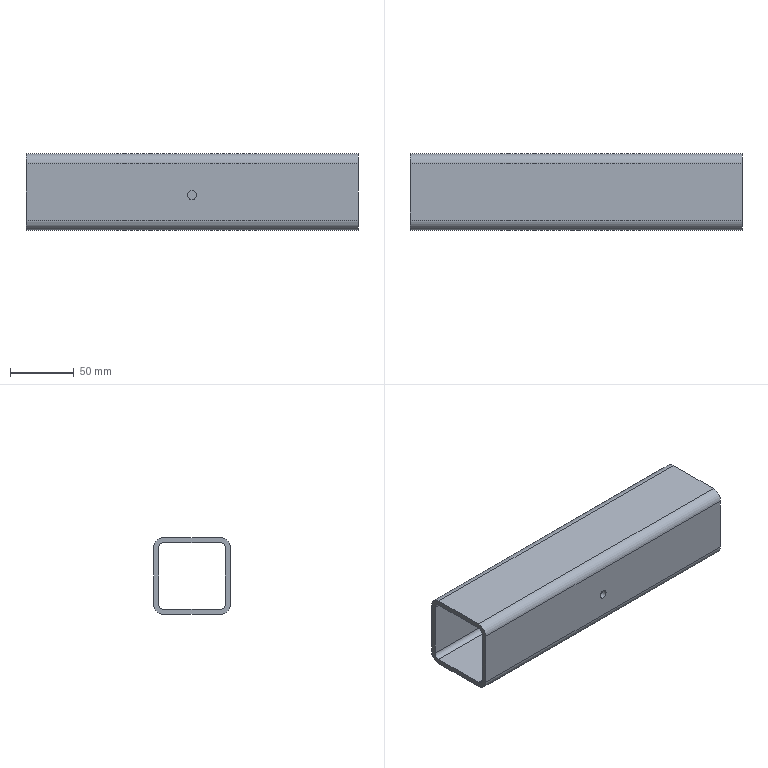Part | SolidWorks | features BaseBody 1 | 1 solid | 20 faces | box 260 x 60 x 60 mm | volume 222102 mm3 | cylinder 10 | plane 10 | commonest cylinder face diameters 8 x4 16 x4 6.8 x2
STEP:
#1=CARTESIAN_POINT('',(-400.,2376.,-1329.1));
#2=VERTEX_POINT('',#1);
#3=CARTESIAN_POINT('',(-400.,2376.,-1335.9));
#4=VERTEX_POINT('',#3);
#5=CARTESIAN_POINT('',(-400.,2376.,-1332.5));
#6=DIRECTION('',(0.,-1.,0.));
#7=DIRECTION('',(0.,0.,-1.));
#8=AXIS2_PLACEMENT_3D('',#5,#6,#7);
#9=CIRCLE('',#8,3.4);
#10=EDGE_CURVE('',#2,#4,#9,.T.);
#11=ORIENTED_EDGE('',*,*,#10,.F.);
#12=CARTESIAN_POINT('',(-400.,2372.,-1329.1));
#13=VERTEX_POINT('',#12);
#14=CARTESIAN_POINT('',(-400.,2362.,-1329.1));
#15=DIRECTION('',(0.,-1.,0.));
#16=VECTOR('',#15,1000.);
#17=LINE('',#14,#16);
#18=EDGE_CURVE('',#2,#13,#17,.T.);
#19=ORIENTED_EDGE('',*,*,#18,.T.);
#20=CARTESIAN_POINT('',(-400.,2372.,-1335.9));
#21=VERTEX_POINT('',#20);
#22=CARTESIAN_POINT('',(-400.,2372.,-1332.5));
#23=DIRECTION('',(0.,-1.,0.));
#24=DIRECTION('',(0.,0.,-1.));
#25=AXIS2_PLACEMENT_3D('',#22,#23,#24);
#26=CIRCLE('',#25,3.4);
#27=EDGE_CURVE('',#13,#21,#26,.T.);
#28=ORIENTED_EDGE('',*,*,#27,.T.);
#29=CARTESIAN_POINT('',(-400.,2362.,-1335.9));
#30=DIRECTION('',(0.,-1.,0.));
#31=VECTOR('',#30,1000.);
#32=LINE('',#29,#31);
#33=EDGE_CURVE('',#4,#21,#32,.T.);
#34=ORIENTED_EDGE('',*,*,#33,.F.);
#35=EDGE_LOOP('',(#11,#19,#28,#34));
#36=FACE_OUTER_BOUND('',#35,.T.);
#37=CARTESIAN_POINT('',(-400.,2362.,-1332.5));
#38=DIRECTION('',(0.,-1.,0.));
#39=DIRECTION('',(0.,0.,-1.));
#40=AXIS2_PLACEMENT_3D('',#37,#38,#39);
#41=CYLINDRICAL_SURFACE('',#40,3.4);
#42=ADVANCED_FACE('',(#36),#41,.F.);
#43=CARTESIAN_POINT('',(-270.,2380.,-1356.));
#44=VERTEX_POINT('',#43);
#45=CARTESIAN_POINT('',(-270.,2424.,-1356.));
#46=VERTEX_POINT('',#45);
#47=CARTESIAN_POINT('',(-270.,2424.,-1356.));
#48=DIRECTION('',(0.,1.,0.));
#49=VECTOR('',#48,1000.);
#50=LINE('',#47,#49);
#51=EDGE_CURVE('',#44,#46,#50,.T.);
#52=ORIENTED_EDGE('',*,*,#51,.T.);
#53=CARTESIAN_POINT('',(-530.,2424.,-1356.));
#54=VERTEX_POINT('',#53);
#55=CARTESIAN_POINT('',(-560.,2424.,-1356.));
#56=DIRECTION('',(-1.,0.,0.));
#57=VECTOR('',#56,1000.);
#58=LINE('',#55,#57);
#59=EDGE_CURVE('',#46,#54,#58,.T.);
#60=ORIENTED_EDGE('',*,*,#59,.T.);
#61=CARTESIAN_POINT('',(-530.,2380.,-1356.));
#62=VERTEX_POINT('',#61);
#63=CARTESIAN_POINT('',(-530.,2424.,-1356.));
#64=DIRECTION('',(0.,-1.,0.));
#65=VECTOR('',#64,1000.);
#66=LINE('',#63,#65);
#67=EDGE_CURVE('',#54,#62,#66,.T.);
#68=ORIENTED_EDGE('',*,*,#67,.T.);
#69=CARTESIAN_POINT('',(-560.,2380.,-1356.));
#70=DIRECTION('',(1.,0.,0.));
#71=VECTOR('',#70,1000.);
#72=LINE('',#69,#71);
#73=EDGE_CURVE('',#62,#44,#72,.T.);
#74=ORIENTED_EDGE('',*,*,#73,.T.);
#75=EDGE_LOOP('',(#52,#60,#68,#74));
#76=FACE_OUTER_BOUND('',#75,.T.);
#77=CARTESIAN_POINT('',(-560.,2424.,-1356.));
#78=DIRECTION('',(0.,0.,1.));
#79=DIRECTION('',(1.,0.,0.));
#80=AXIS2_PLACEMENT_3D('',#77,#78,#79);
#81=PLANE('',#80);
#82=ADVANCED_FACE('',(#76),#81,.T.);
#83=ORIENTED_EDGE('',*,*,#59,.F.);
#84=CARTESIAN_POINT('',(-270.,2428.,-1352.));
#85=VERTEX_POINT('',#84);
#86=CARTESIAN_POINT('',(-270.,2424.,-1352.));
#87=DIRECTION('',(-1.,0.,0.));
#88=DIRECTION('',(0.,0.,-1.));
#89=AXIS2_PLACEMENT_3D('',#86,#87,#88);
#90=CIRCLE('',#89,4.);
#91=EDGE_CURVE('',#85,#46,#90,.T.);
#92=ORIENTED_EDGE('',*,*,#91,.F.);
#93=CARTESIAN_POINT('',(-530.,2428.,-1352.));
#94=VERTEX_POINT('',#93);
#95=CARTESIAN_POINT('',(-560.,2428.,-1352.));
#96=DIRECTION('',(1.,0.,0.));
#97=VECTOR('',#96,1000.);
#98=LINE('',#95,#97);
#99=EDGE_CURVE('',#94,#85,#98,.T.);
#100=ORIENTED_EDGE('',*,*,#99,.F.);
#101=CARTESIAN_POINT('',(-530.,2424.,-1352.));
#102=DIRECTION('',(1.,0.,0.));
#103=DIRECTION('',(0.,0.,-1.));
#104=AXIS2_PLACEMENT_3D('',#101,#102,#103);
#105=CIRCLE('',#104,4.);
#106=EDGE_CURVE('',#54,#94,#105,.T.);
#107=ORIENTED_EDGE('',*,*,#106,.F.);
#108=EDGE_LOOP('',(#83,#92,#100,#107));
#109=FACE_OUTER_BOUND('',#108,.T.);
#110=CARTESIAN_POINT('',(-560.,2424.,-1352.));
#111=DIRECTION('',(1.,0.,0.));
#112=DIRECTION('',(0.,0.,-1.));
#113=AXIS2_PLACEMENT_3D('',#110,#111,#112);
#114=CYLINDRICAL_SURFACE('',#113,4.);
#115=ADVANCED_FACE('',(#109),#114,.F.);
#116=CARTESIAN_POINT('',(-270.,2376.,-1352.));
#117=VERTEX_POINT('',#116);
#118=CARTESIAN_POINT('',(-270.,2380.,-1352.));
#119=DIRECTION('',(-1.,0.,0.));
#120=DIRECTION('',(0.,0.,-1.));
#121=AXIS2_PLACEMENT_3D('',#118,#119,#120);
#122=CIRCLE('',#121,4.);
#123=EDGE_CURVE('',#44,#117,#122,.T.);
#124=ORIENTED_EDGE('',*,*,#123,.T.);
#125=CARTESIAN_POINT('',(-270.,2376.,-1308.));
#126=VERTEX_POINT('',#125);
#127=CARTESIAN_POINT('',(-270.,2376.,-1352.));
#128=DIRECTION('',(0.,0.,1.));
#129=VECTOR('',#128,1000.);
#130=LINE('',#127,#129);
#131=EDGE_CURVE('',#117,#126,#130,.T.);
#132=ORIENTED_EDGE('',*,*,#131,.T.);
#133=CARTESIAN_POINT('',(-270.,2380.,-1304.));
#134=VERTEX_POINT('',#133);
#135=CARTESIAN_POINT('',(-270.,2380.,-1308.));
#136=DIRECTION('',(-1.,0.,0.));
#137=DIRECTION('',(0.,0.,-1.));
#138=AXIS2_PLACEMENT_3D('',#135,#136,#137);
#139=CIRCLE('',#138,4.);
#140=EDGE_CURVE('',#126,#134,#139,.T.);
#141=ORIENTED_EDGE('',*,*,#140,.T.);
#142=CARTESIAN_POINT('',(-270.,2424.,-1304.));
#143=VERTEX_POINT('',#142);
#144=CARTESIAN_POINT('',(-270.,102.,-1304.));
#145=DIRECTION('',(0.,1.,0.));
#146=VECTOR('',#145,1000.);
#147=LINE('',#144,#146);
#148=EDGE_CURVE('',#134,#143,#147,.T.);
#149=ORIENTED_EDGE('',*,*,#148,.T.);
#150=CARTESIAN_POINT('',(-270.,2428.,-1308.));
#151=VERTEX_POINT('',#150);
#152=CARTESIAN_POINT('',(-270.,2424.,-1308.));
#153=DIRECTION('',(-1.,0.,0.));
#154=DIRECTION('',(0.,0.,-1.));
#155=AXIS2_PLACEMENT_3D('',#152,#153,#154);
#156=CIRCLE('',#155,4.);
#157=EDGE_CURVE('',#143,#151,#156,.T.);
#158=ORIENTED_EDGE('',*,*,#157,.T.);
#159=CARTESIAN_POINT('',(-270.,2428.,-1352.));
#160=DIRECTION('',(0.,0.,-1.));
#161=VECTOR('',#160,1000.);
#162=LINE('',#159,#161);
#163=EDGE_CURVE('',#151,#85,#162,.T.);
#164=ORIENTED_EDGE('',*,*,#163,.T.);
#165=ORIENTED_EDGE('',*,*,#91,.T.);
#166=ORIENTED_EDGE('',*,*,#51,.F.);
#167=EDGE_LOOP('',(#124,#132,#141,#149,#158,#164,#165,#166));
#168=FACE_BOUND('',#167,.T.);
#169=CARTESIAN_POINT('',(-270.,2372.,-1308.));
#170=VERTEX_POINT('',#169);
#171=CARTESIAN_POINT('',(-270.,2372.,-1352.));
#172=VERTEX_POINT('',#171);
#173=CARTESIAN_POINT('',(-270.,2372.,-1352.));
#174=DIRECTION('',(0.,0.,-1.));
#175=VECTOR('',#174,1000.);
#176=LINE('',#173,#175);
#177=EDGE_CURVE('',#170,#172,#176,.T.);
#178=ORIENTED_EDGE('',*,*,#177,.T.);
#179=CARTESIAN_POINT('',(-270.,2380.,-1360.));
#180=VERTEX_POINT('',#179);
#181=CARTESIAN_POINT('',(-270.,2380.,-1352.));
#182=DIRECTION('',(1.,0.,0.));
#183=DIRECTION('',(0.,0.,-1.));
#184=AXIS2_PLACEMENT_3D('',#181,#182,#183);
#185=CIRCLE('',#184,8.);
#186=EDGE_CURVE('',#172,#180,#185,.T.);
#187=ORIENTED_EDGE('',*,*,#186,.T.);
#188=CARTESIAN_POINT('',(-270.,2424.,-1360.));
#189=VERTEX_POINT('',#188);
#190=CARTESIAN_POINT('',(-270.,102.,-1360.));
#191=DIRECTION('',(0.,1.,0.));
#192=VECTOR('',#191,1000.);
#193=LINE('',#190,#192);
#194=EDGE_CURVE('',#180,#189,#193,.T.);
#195=ORIENTED_EDGE('',*,*,#194,.T.);
#196=CARTESIAN_POINT('',(-270.,2432.,-1352.));
#197=VERTEX_POINT('',#196);
#198=CARTESIAN_POINT('',(-270.,2424.,-1352.));
#199=DIRECTION('',(1.,0.,0.));
#200=DIRECTION('',(0.,0.,-1.));
#201=AXIS2_PLACEMENT_3D('',#198,#199,#200);
#202=CIRCLE('',#201,8.);
#203=EDGE_CURVE('',#189,#197,#202,.T.);
#204=ORIENTED_EDGE('',*,*,#203,.T.);
#205=CARTESIAN_POINT('',(-270.,2432.,-1308.));
#206=VERTEX_POINT('',#205);
#207=CARTESIAN_POINT('',(-270.,2432.,-1352.));
#208=DIRECTION('',(0.,0.,1.));
#209=VECTOR('',#208,1000.);
#210=LINE('',#207,#209);
#211=EDGE_CURVE('',#197,#206,#210,.T.);
#212=ORIENTED_EDGE('',*,*,#211,.T.);
#213=CARTESIAN_POINT('',(-270.,2424.,-1300.));
#214=VERTEX_POINT('',#213);
#215=CARTESIAN_POINT('',(-270.,2424.,-1308.));
#216=DIRECTION('',(1.,0.,0.));
#217=DIRECTION('',(0.,0.,-1.));
#218=AXIS2_PLACEMENT_3D('',#215,#216,#217);
#219=CIRCLE('',#218,8.);
#220=EDGE_CURVE('',#206,#214,#219,.T.);
#221=ORIENTED_EDGE('',*,*,#220,.T.);
#222=CARTESIAN_POINT('',(-270.,2380.,-1300.));
#223=VERTEX_POINT('',#222);
#224=CARTESIAN_POINT('',(-270.,102.,-1300.));
#225=DIRECTION('',(0.,-1.,0.));
#226=VECTOR('',#225,1000.);
#227=LINE('',#224,#226);
#228=EDGE_CURVE('',#214,#223,#227,.T.);
#229=ORIENTED_EDGE('',*,*,#228,.T.);
#230=CARTESIAN_POINT('',(-270.,2380.,-1308.));
#231=DIRECTION('',(1.,0.,0.));
#232=DIRECTION('',(0.,0.,-1.));
#233=AXIS2_PLACEMENT_3D('',#230,#231,#232);
#234=CIRCLE('',#233,8.);
#235=EDGE_CURVE('',#223,#170,#234,.T.);
#236=ORIENTED_EDGE('',*,*,#235,.T.);
#237=EDGE_LOOP('',(#178,#187,#195,#204,#212,#221,#229,#236));
#238=FACE_OUTER_BOUND('',#237,.T.);
#239=CARTESIAN_POINT('',(-270.,102.,-1352.));
#240=DIRECTION('',(1.,0.,0.));
#241=DIRECTION('',(0.,0.,-1.));
#242=AXIS2_PLACEMENT_3D('',#239,#240,#241);
#243=PLANE('',#242);
#244=ADVANCED_FACE('',(#168,#238),#243,.T.);
#245=CARTESIAN_POINT('',(-530.,2376.,-1352.));
#246=VERTEX_POINT('',#245);
#247=CARTESIAN_POINT('',(-560.,2376.,-1352.));
#248=DIRECTION('',(-1.,0.,0.));
#249=VECTOR('',#248,1000.);
#250=LINE('',#247,#249);
#251=EDGE_CURVE('',#117,#246,#250,.T.);
#252=ORIENTED_EDGE('',*,*,#251,.F.);
#253=ORIENTED_EDGE('',*,*,#123,.F.);
#254=ORIENTED_EDGE('',*,*,#73,.F.);
#255=CARTESIAN_POINT('',(-530.,2380.,-1352.));
#256=DIRECTION('',(1.,0.,0.));
#257=DIRECTION('',(0.,0.,-1.));
#258=AXIS2_PLACEMENT_3D('',#255,#256,#257);
#259=CIRCLE('',#258,4.);
#260=EDGE_CURVE('',#246,#62,#259,.T.);
#261=ORIENTED_EDGE('',*,*,#260,.F.);
#262=EDGE_LOOP('',(#252,#253,#254,#261));
#263=FACE_OUTER_BOUND('',#262,.T.);
#264=CARTESIAN_POINT('',(-560.,2380.,-1352.));
#265=DIRECTION('',(1.,0.,0.));
#266=DIRECTION('',(0.,0.,-1.));
#267=AXIS2_PLACEMENT_3D('',#264,#265,#266);
#268=CYLINDRICAL_SURFACE('',#267,4.);
#269=ADVANCED_FACE('',(#263),#268,.F.);
#270=ORIENTED_EDGE('',*,*,#260,.T.);
#271=ORIENTED_EDGE('',*,*,#67,.F.);
#272=ORIENTED_EDGE('',*,*,#106,.T.);
#273=CARTESIAN_POINT('',(-530.,2428.,-1308.));
#274=VERTEX_POINT('',#273);
#275=CARTESIAN_POINT('',(-530.,2428.,-1308.));
#276=DIRECTION('',(0.,0.,1.));
#277=VECTOR('',#276,1000.);
#278=LINE('',#275,#277);
#279=EDGE_CURVE('',#94,#274,#278,.T.);
#280=ORIENTED_EDGE('',*,*,#279,.T.);
#281=CARTESIAN_POINT('',(-530.,2424.,-1304.));
#282=VERTEX_POINT('',#281);
#283=CARTESIAN_POINT('',(-530.,2424.,-1308.));
#284=DIRECTION('',(1.,0.,0.));
#285=DIRECTION('',(0.,0.,-1.));
#286=AXIS2_PLACEMENT_3D('',#283,#284,#285);
#287=CIRCLE('',#286,4.);
#288=EDGE_CURVE('',#274,#282,#287,.T.);
#289=ORIENTED_EDGE('',*,*,#288,.T.);
#290=CARTESIAN_POINT('',(-530.,2380.,-1304.));
#291=VERTEX_POINT('',#290);
#292=CARTESIAN_POINT('',(-530.,102.,-1304.));
#293=DIRECTION('',(0.,-1.,0.));
#294=VECTOR('',#293,1000.);
#295=LINE('',#292,#294);
#296=EDGE_CURVE('',#282,#291,#295,.T.);
#297=ORIENTED_EDGE('',*,*,#296,.T.);
#298=CARTESIAN_POINT('',(-530.,2376.,-1308.));
#299=VERTEX_POINT('',#298);
#300=CARTESIAN_POINT('',(-530.,2380.,-1308.));
#301=DIRECTION('',(1.,0.,0.));
#302=DIRECTION('',(0.,0.,-1.));
#303=AXIS2_PLACEMENT_3D('',#300,#301,#302);
#304=CIRCLE('',#303,4.);
#305=EDGE_CURVE('',#291,#299,#304,.T.);
#306=ORIENTED_EDGE('',*,*,#305,.T.);
#307=CARTESIAN_POINT('',(-530.,2376.,-1308.));
#308=DIRECTION('',(0.,0.,-1.));
#309=VECTOR('',#308,1000.);
#310=LINE('',#307,#309);
#311=EDGE_CURVE('',#299,#246,#310,.T.);
#312=ORIENTED_EDGE('',*,*,#311,.T.);
#313=EDGE_LOOP('',(#270,#271,#272,#280,#289,#297,#306,#312));
#314=FACE_BOUND('',#313,.T.);
#315=CARTESIAN_POINT('',(-530.,2424.,-1360.));
#316=VERTEX_POINT('',#315);
#317=CARTESIAN_POINT('',(-530.,2380.,-1360.));
#318=VERTEX_POINT('',#317);
#319=CARTESIAN_POINT('',(-530.,102.,-1360.));
#320=DIRECTION('',(0.,-1.,0.));
#321=VECTOR('',#320,1000.);
#322=LINE('',#319,#321);
#323=EDGE_CURVE('',#316,#318,#322,.T.);
#324=ORIENTED_EDGE('',*,*,#323,.T.);
#325=CARTESIAN_POINT('',(-530.,2372.,-1352.));
#326=VERTEX_POINT('',#325);
#327=CARTESIAN_POINT('',(-530.,2380.,-1352.));
#328=DIRECTION('',(-1.,0.,0.));
#329=DIRECTION('',(0.,0.,-1.));
#330=AXIS2_PLACEMENT_3D('',#327,#328,#329);
#331=CIRCLE('',#330,8.);
#332=EDGE_CURVE('',#318,#326,#331,.T.);
#333=ORIENTED_EDGE('',*,*,#332,.T.);
#334=CARTESIAN_POINT('',(-530.,2372.,-1308.));
#335=VERTEX_POINT('',#334);
#336=CARTESIAN_POINT('',(-530.,2372.,-1308.));
#337=DIRECTION('',(0.,0.,1.));
#338=VECTOR('',#337,1000.);
#339=LINE('',#336,#338);
#340=EDGE_CURVE('',#326,#335,#339,.T.);
#341=ORIENTED_EDGE('',*,*,#340,.T.);
#342=CARTESIAN_POINT('',(-530.,2380.,-1300.));
#343=VERTEX_POINT('',#342);
#344=CARTESIAN_POINT('',(-530.,2380.,-1308.));
#345=DIRECTION('',(-1.,0.,0.));
#346=DIRECTION('',(0.,0.,-1.));
#347=AXIS2_PLACEMENT_3D('',#344,#345,#346);
#348=CIRCLE('',#347,8.);
#349=EDGE_CURVE('',#335,#343,#348,.T.);
#350=ORIENTED_EDGE('',*,*,#349,.T.);
#351=CARTESIAN_POINT('',(-530.,2424.,-1300.));
#352=VERTEX_POINT('',#351);
#353=CARTESIAN_POINT('',(-530.,102.,-1300.));
#354=DIRECTION('',(0.,1.,0.));
#355=VECTOR('',#354,1000.);
#356=LINE('',#353,#355);
#357=EDGE_CURVE('',#343,#352,#356,.T.);
#358=ORIENTED_EDGE('',*,*,#357,.T.);
#359=CARTESIAN_POINT('',(-530.,2432.,-1308.));
#360=VERTEX_POINT('',#359);
#361=CARTESIAN_POINT('',(-530.,2424.,-1308.));
#362=DIRECTION('',(-1.,0.,0.));
#363=DIRECTION('',(0.,0.,-1.));
#364=AXIS2_PLACEMENT_3D('',#361,#362,#363);
#365=CIRCLE('',#364,8.);
#366=EDGE_CURVE('',#352,#360,#365,.T.);
#367=ORIENTED_EDGE('',*,*,#366,.T.);
#368=CARTESIAN_POINT('',(-530.,2432.,-1352.));
#369=VERTEX_POINT('',#368);
#370=CARTESIAN_POINT('',(-530.,2432.,-1308.));
#371=DIRECTION('',(0.,0.,-1.));
#372=VECTOR('',#371,1000.);
#373=LINE('',#370,#372);
#374=EDGE_CURVE('',#360,#369,#373,.T.);
#375=ORIENTED_EDGE('',*,*,#374,.T.);
#376=CARTESIAN_POINT('',(-530.,2424.,-1352.));
#377=DIRECTION('',(-1.,0.,0.));
#378=DIRECTION('',(0.,0.,-1.));
#379=AXIS2_PLACEMENT_3D('',#376,#377,#378);
#380=CIRCLE('',#379,8.);
#381=EDGE_CURVE('',#369,#316,#380,.T.);
#382=ORIENTED_EDGE('',*,*,#381,.T.);
#383=EDGE_LOOP('',(#324,#333,#341,#350,#358,#367,#375,#382));
#384=FACE_OUTER_BOUND('',#383,.T.);
#385=CARTESIAN_POINT('',(-530.,102.,-1308.));
#386=DIRECTION('',(-1.,0.,0.));
#387=DIRECTION('',(0.,0.,1.));
#388=AXIS2_PLACEMENT_3D('',#385,#386,#387);
#389=PLANE('',#388);
#390=ADVANCED_FACE('',(#314,#384),#389,.T.);
#391=ORIENTED_EDGE('',*,*,#163,.F.);
#392=CARTESIAN_POINT('',(-560.,2428.,-1308.));
#393=DIRECTION('',(-1.,0.,0.));
#394=VECTOR('',#393,1000.);
#395=LINE('',#392,#394);
#396=EDGE_CURVE('',#151,#274,#395,.T.);
#397=ORIENTED_EDGE('',*,*,#396,.T.);
#398=ORIENTED_EDGE('',*,*,#279,.F.);
#399=ORIENTED_EDGE('',*,*,#99,.T.);
#400=EDGE_LOOP('',(#391,#397,#398,#399));
#401=FACE_OUTER_BOUND('',#400,.T.);
#402=CARTESIAN_POINT('',(-560.,2428.,-1352.));
#403=DIRECTION('',(0.,-1.,0.));
#404=DIRECTION('',(0.,0.,-1.));
#405=AXIS2_PLACEMENT_3D('',#402,#403,#404);
#406=PLANE('',#405);
#407=ADVANCED_FACE('',(#401),#406,.T.);
#408=CARTESIAN_POINT('',(-400.,2376.,-1332.5));
#409=DIRECTION('',(0.,-1.,0.));
#410=DIRECTION('',(0.,0.,-1.));
#411=AXIS2_PLACEMENT_3D('',#408,#409,#410);
#412=CIRCLE('',#411,3.4);
#413=EDGE_CURVE('',#4,#2,#412,.T.);
#414=ORIENTED_EDGE('',*,*,#413,.T.);
#415=ORIENTED_EDGE('',*,*,#10,.T.);
#416=EDGE_LOOP('',(#414,#415));
#417=FACE_BOUND('',#416,.T.);
#418=ORIENTED_EDGE('',*,*,#131,.F.);
#419=ORIENTED_EDGE('',*,*,#251,.T.);
#420=ORIENTED_EDGE('',*,*,#311,.F.);
#421=CARTESIAN_POINT('',(-560.,2376.,-1308.));
#422=DIRECTION('',(1.,0.,0.));
#423=VECTOR('',#422,1000.);
#424=LINE('',#421,#423);
#425=EDGE_CURVE('',#299,#126,#424,.T.);
#426=ORIENTED_EDGE('',*,*,#425,.T.);
#427=EDGE_LOOP('',(#418,#419,#420,#426));
#428=FACE_OUTER_BOUND('',#427,.T.);
#429=CARTESIAN_POINT('',(-560.,2376.,-1308.));
#430=DIRECTION('',(0.,1.,0.));
#431=DIRECTION('',(0.,0.,1.));
#432=AXIS2_PLACEMENT_3D('',#429,#430,#431);
#433=PLANE('',#432);
#434=ADVANCED_FACE('',(#417,#428),#433,.T.);
#435=ORIENTED_EDGE('',*,*,#396,.F.);
#436=ORIENTED_EDGE('',*,*,#157,.F.);
#437=CARTESIAN_POINT('',(-560.,2424.,-1304.));
#438=DIRECTION('',(1.,0.,0.));
#439=VECTOR('',#438,1000.);
#440=LINE('',#437,#439);
#441=EDGE_CURVE('',#282,#143,#440,.T.);
#442=ORIENTED_EDGE('',*,*,#441,.F.);
#443=ORIENTED_EDGE('',*,*,#288,.F.);
#444=EDGE_LOOP('',(#435,#436,#442,#443));
#445=FACE_OUTER_BOUND('',#444,.T.);
#446=CARTESIAN_POINT('',(-560.,2424.,-1308.));
#447=DIRECTION('',(1.,0.,0.));
#448=DIRECTION('',(0.,0.,-1.));
#449=AXIS2_PLACEMENT_3D('',#446,#447,#448);
#450=CYLINDRICAL_SURFACE('',#449,4.);
#451=ADVANCED_FACE('',(#445),#450,.F.);
#452=ORIENTED_EDGE('',*,*,#148,.F.);
#453=CARTESIAN_POINT('',(-560.,2380.,-1304.));
#454=DIRECTION('',(-1.,0.,0.));
#455=VECTOR('',#454,1000.);
#456=LINE('',#453,#455);
#457=EDGE_CURVE('',#134,#291,#456,.T.);
#458=ORIENTED_EDGE('',*,*,#457,.T.);
#459=ORIENTED_EDGE('',*,*,#296,.F.);
#460=ORIENTED_EDGE('',*,*,#441,.T.);
#461=EDGE_LOOP('',(#452,#458,#459,#460));
#462=FACE_OUTER_BOUND('',#461,.T.);
#463=CARTESIAN_POINT('',(-560.,2380.,-1304.));
#464=DIRECTION('',(0.,0.,-1.));
#465=DIRECTION('',(-1.,0.,0.));
#466=AXIS2_PLACEMENT_3D('',#463,#464,#465);
#467=PLANE('',#466);
#468=ADVANCED_FACE('',(#462),#467,.T.);
#469=ORIENTED_EDGE('',*,*,#457,.F.);
#470=ORIENTED_EDGE('',*,*,#140,.F.);
#471=ORIENTED_EDGE('',*,*,#425,.F.);
#472=ORIENTED_EDGE('',*,*,#305,.F.);
#473=EDGE_LOOP('',(#469,#470,#471,#472));
#474=FACE_OUTER_BOUND('',#473,.T.);
#475=CARTESIAN_POINT('',(-560.,2380.,-1308.));
#476=DIRECTION('',(1.,0.,0.));
#477=DIRECTION('',(0.,0.,-1.));
#478=AXIS2_PLACEMENT_3D('',#475,#476,#477);
#479=CYLINDRICAL_SURFACE('',#478,4.);
#480=ADVANCED_FACE('',(#474),#479,.F.);
#481=CARTESIAN_POINT('',(-560.,2372.,-1352.));
#482=DIRECTION('',(-1.,0.,0.));
#483=VECTOR('',#482,1000.);
#484=LINE('',#481,#483);
#485=EDGE_CURVE('',#172,#326,#484,.T.);
#486=ORIENTED_EDGE('',*,*,#485,.T.);
#487=ORIENTED_EDGE('',*,*,#332,.F.);
#488=CARTESIAN_POINT('',(-560.,2380.,-1360.));
#489=DIRECTION('',(1.,0.,0.));
#490=VECTOR('',#489,1000.);
#491=LINE('',#488,#490);
#492=EDGE_CURVE('',#318,#180,#491,.T.);
#493=ORIENTED_EDGE('',*,*,#492,.T.);
#494=ORIENTED_EDGE('',*,*,#186,.F.);
#495=EDGE_LOOP('',(#486,#487,#493,#494));
#496=FACE_OUTER_BOUND('',#495,.T.);
#497=CARTESIAN_POINT('',(-560.,2380.,-1352.));
#498=DIRECTION('',(1.,0.,0.));
#499=DIRECTION('',(0.,0.,-1.));
#500=AXIS2_PLACEMENT_3D('',#497,#498,#499);
#501=CYLINDRICAL_SURFACE('',#500,8.);
#502=ADVANCED_FACE('',(#496),#501,.T.);
#503=CARTESIAN_POINT('',(-400.,2372.,-1332.5));
#504=DIRECTION('',(0.,-1.,0.));
#505=DIRECTION('',(0.,0.,-1.));
#506=AXIS2_PLACEMENT_3D('',#503,#504,#505);
#507=CIRCLE('',#506,3.4);
#508=EDGE_CURVE('',#21,#13,#507,.T.);
#509=ORIENTED_EDGE('',*,*,#508,.F.);
#510=ORIENTED_EDGE('',*,*,#27,.F.);
#511=EDGE_LOOP('',(#509,#510));
#512=FACE_BOUND('',#511,.T.);
#513=ORIENTED_EDGE('',*,*,#177,.F.);
#514=CARTESIAN_POINT('',(-560.,2372.,-1308.));
#515=DIRECTION('',(1.,0.,0.));
#516=VECTOR('',#515,1000.);
#517=LINE('',#514,#516);
#518=EDGE_CURVE('',#335,#170,#517,.T.);
#519=ORIENTED_EDGE('',*,*,#518,.F.);
#520=ORIENTED_EDGE('',*,*,#340,.F.);
#521=ORIENTED_EDGE('',*,*,#485,.F.);
#522=EDGE_LOOP('',(#513,#519,#520,#521));
#523=FACE_OUTER_BOUND('',#522,.T.);
#524=CARTESIAN_POINT('',(-560.,2372.,-1308.));
#525=DIRECTION('',(0.,1.,0.));
#526=DIRECTION('',(0.,0.,1.));
#527=AXIS2_PLACEMENT_3D('',#524,#525,#526);
#528=PLANE('',#527);
#529=ADVANCED_FACE('',(#512,#523),#528,.F.);
#530=CARTESIAN_POINT('',(-560.,2380.,-1300.));
#531=DIRECTION('',(-1.,0.,0.));
#532=VECTOR('',#531,1000.);
#533=LINE('',#530,#532);
#534=EDGE_CURVE('',#223,#343,#533,.T.);
#535=ORIENTED_EDGE('',*,*,#534,.T.);
#536=ORIENTED_EDGE('',*,*,#349,.F.);
#537=ORIENTED_EDGE('',*,*,#518,.T.);
#538=ORIENTED_EDGE('',*,*,#235,.F.);
#539=EDGE_LOOP('',(#535,#536,#537,#538));
#540=FACE_OUTER_BOUND('',#539,.T.);
#541=CARTESIAN_POINT('',(-560.,2380.,-1308.));
#542=DIRECTION('',(1.,0.,0.));
#543=DIRECTION('',(0.,0.,-1.));
#544=AXIS2_PLACEMENT_3D('',#541,#542,#543);
#545=CYLINDRICAL_SURFACE('',#544,8.);
#546=ADVANCED_FACE('',(#540),#545,.T.);
#547=ORIENTED_EDGE('',*,*,#228,.F.);
#548=CARTESIAN_POINT('',(-560.,2424.,-1300.));
#549=DIRECTION('',(1.,0.,0.));
#550=VECTOR('',#549,1000.);
#551=LINE('',#548,#550);
#552=EDGE_CURVE('',#352,#214,#551,.T.);
#553=ORIENTED_EDGE('',*,*,#552,.F.);
#554=ORIENTED_EDGE('',*,*,#357,.F.);
#555=ORIENTED_EDGE('',*,*,#534,.F.);
#556=EDGE_LOOP('',(#547,#553,#554,#555));
#557=FACE_OUTER_BOUND('',#556,.T.);
#558=CARTESIAN_POINT('',(-560.,2380.,-1300.));
#559=DIRECTION('',(0.,0.,-1.));
#560=DIRECTION('',(-1.,0.,0.));
#561=AXIS2_PLACEMENT_3D('',#558,#559,#560);
#562=PLANE('',#561);
#563=ADVANCED_FACE('',(#557),#562,.F.);
#564=CARTESIAN_POINT('',(-560.,2432.,-1308.));
#565=DIRECTION('',(-1.,0.,0.));
#566=VECTOR('',#565,1000.);
#567=LINE('',#564,#566);
#568=EDGE_CURVE('',#206,#360,#567,.T.);
#569=ORIENTED_EDGE('',*,*,#568,.T.);
#570=ORIENTED_EDGE('',*,*,#366,.F.);
#571=ORIENTED_EDGE('',*,*,#552,.T.);
#572=ORIENTED_EDGE('',*,*,#220,.F.);
#573=EDGE_LOOP('',(#569,#570,#571,#572));
#574=FACE_OUTER_BOUND('',#573,.T.);
#575=CARTESIAN_POINT('',(-560.,2424.,-1308.));
#576=DIRECTION('',(1.,0.,0.));
#577=DIRECTION('',(0.,0.,-1.));
#578=AXIS2_PLACEMENT_3D('',#575,#576,#577);
#579=CYLINDRICAL_SURFACE('',#578,8.);
#580=ADVANCED_FACE('',(#574),#579,.T.);
#581=ORIENTED_EDGE('',*,*,#211,.F.);
#582=CARTESIAN_POINT('',(-560.,2432.,-1352.));
#583=DIRECTION('',(1.,0.,0.));
#584=VECTOR('',#583,1000.);
#585=LINE('',#582,#584);
#586=EDGE_CURVE('',#369,#197,#585,.T.);
#587=ORIENTED_EDGE('',*,*,#586,.F.);
#588=ORIENTED_EDGE('',*,*,#374,.F.);
#589=ORIENTED_EDGE('',*,*,#568,.F.);
#590=EDGE_LOOP('',(#581,#587,#588,#589));
#591=FACE_OUTER_BOUND('',#590,.T.);
#592=CARTESIAN_POINT('',(-560.,2432.,-1352.));
#593=DIRECTION('',(0.,-1.,0.));
#594=DIRECTION('',(0.,0.,-1.));
#595=AXIS2_PLACEMENT_3D('',#592,#593,#594);
#596=PLANE('',#595);
#597=ADVANCED_FACE('',(#591),#596,.F.);
#598=CARTESIAN_POINT('',(-560.,2424.,-1360.));
#599=DIRECTION('',(-1.,0.,0.));
#600=VECTOR('',#599,1000.);
#601=LINE('',#598,#600);
#602=EDGE_CURVE('',#189,#316,#601,.T.);
#603=ORIENTED_EDGE('',*,*,#602,.T.);
#604=ORIENTED_EDGE('',*,*,#381,.F.);
#605=ORIENTED_EDGE('',*,*,#586,.T.);
#606=ORIENTED_EDGE('',*,*,#203,.F.);
#607=EDGE_LOOP('',(#603,#604,#605,#606));
#608=FACE_OUTER_BOUND('',#607,.T.);
#609=CARTESIAN_POINT('',(-560.,2424.,-1352.));
#610=DIRECTION('',(1.,0.,0.));
#611=DIRECTION('',(0.,0.,-1.));
#612=AXIS2_PLACEMENT_3D('',#609,#610,#611);
#613=CYLINDRICAL_SURFACE('',#612,8.);
#614=ADVANCED_FACE('',(#608),#613,.T.);
#615=ORIENTED_EDGE('',*,*,#194,.F.);
#616=ORIENTED_EDGE('',*,*,#492,.F.);
#617=ORIENTED_EDGE('',*,*,#323,.F.);
#618=ORIENTED_EDGE('',*,*,#602,.F.);
#619=EDGE_LOOP('',(#615,#616,#617,#618));
#620=FACE_OUTER_BOUND('',#619,.T.);
#621=CARTESIAN_POINT('',(-560.,2424.,-1360.));
#622=DIRECTION('',(0.,0.,1.));
#623=DIRECTION('',(1.,0.,0.));
#624=AXIS2_PLACEMENT_3D('',#621,#622,#623);
#625=PLANE('',#624);
#626=ADVANCED_FACE('',(#620),#625,.F.);
#627=ORIENTED_EDGE('',*,*,#18,.F.);
#628=ORIENTED_EDGE('',*,*,#413,.F.);
#629=ORIENTED_EDGE('',*,*,#33,.T.);
#630=ORIENTED_EDGE('',*,*,#508,.T.);
#631=EDGE_LOOP('',(#627,#628,#629,#630));
#632=FACE_OUTER_BOUND('',#631,.T.);
#633=CARTESIAN_POINT('',(-400.,2362.,-1332.5));
#634=DIRECTION('',(0.,-1.,0.));
#635=DIRECTION('',(0.,0.,-1.));
#636=AXIS2_PLACEMENT_3D('',#633,#634,#635);
#637=CYLINDRICAL_SURFACE('',#636,3.4);
#638=ADVANCED_FACE('',(#632),#637,.F.);
#639=CLOSED_SHELL('',(#42,#82,#115,#244,#269,#390,#407,#434,#451,#468,#480,#502,#529,#546,#563,#580,#597,#614,#626,#638));
#640=MANIFOLD_SOLID_BREP('',#639);
#641=CARTESIAN_POINT('',(0.,0.,0.));
#642=DIRECTION('',(0.,0.,1.));
#643=DIRECTION('',(1.,0.,0.));
#644=AXIS2_PLACEMENT_3D('',#641,#642,#643);
#645=(LENGTH_UNIT()NAMED_UNIT(*)SI_UNIT(.MILLI.,.METRE.));
#646=UNCERTAINTY_MEASURE_WITH_UNIT(LENGTH_MEASURE(0.00001),#645,'','');
#647=(NAMED_UNIT(*)PLANE_ANGLE_UNIT()SI_UNIT($,.RADIAN.));
#648=(NAMED_UNIT(*)SI_UNIT($,.STERADIAN.)SOLID_ANGLE_UNIT());
#649=(GEOMETRIC_REPRESENTATION_CONTEXT(3)GLOBAL_UNCERTAINTY_ASSIGNED_CONTEXT((#646))GLOBAL_UNIT_ASSIGNED_CONTEXT((#645,#647,#648))REPRESENTATION_CONTEXT('',''));
#650=ADVANCED_BREP_SHAPE_REPRESENTATION('',(#640,#644),#649);